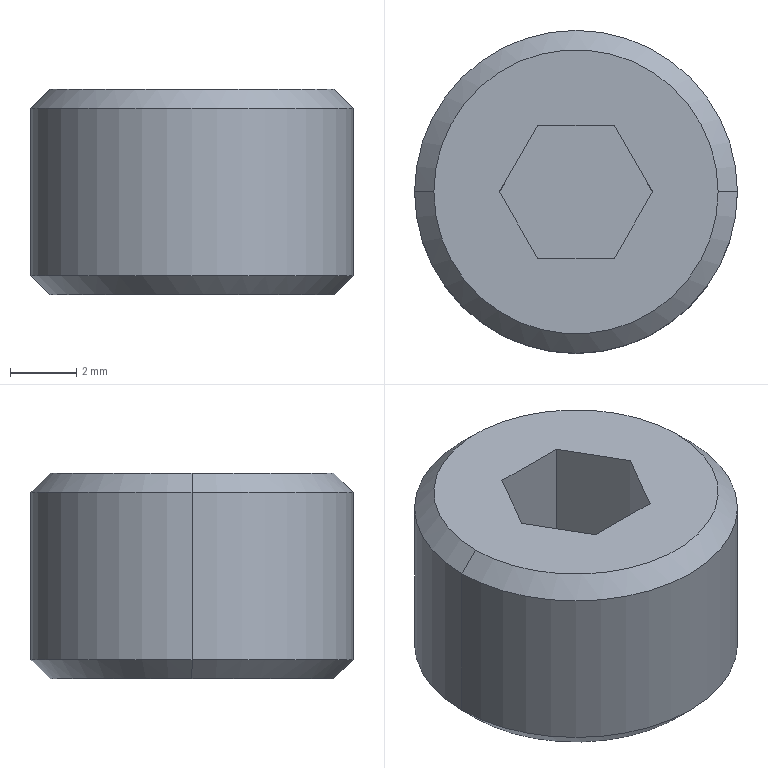Part | SolidWorks | features BaseBody 1 | 1 solid | 15 faces | box 9.728 x 9.728 x 6.2 mm | volume 395.486 mm3 | plane 9 | cone 4 | cylinder 2 | commonest cylinder face diameters 9.728 x2
STEP:
#1=CARTESIAN_POINT('',(-4.283,0.,-6.2));
#2=VERTEX_POINT('',#1);
#3=CARTESIAN_POINT('',(4.283,0.,-6.2));
#4=VERTEX_POINT('',#3);
#5=CARTESIAN_POINT('',(0.,0.,-6.2));
#6=DIRECTION('',(0.,0.,-1.));
#7=DIRECTION('',(-1.,0.,0.));
#8=AXIS2_PLACEMENT_3D('',#5,#6,#7);
#9=CIRCLE('',#8,4.283);
#10=EDGE_CURVE('',#2,#4,#9,.T.);
#11=ORIENTED_EDGE('',*,*,#10,.F.);
#12=CARTESIAN_POINT('',(-4.864,0.,-5.619));
#13=VERTEX_POINT('',#12);
#14=CARTESIAN_POINT('',(-4.864,0.,-5.619));
#15=DIRECTION('',(-0.7071,0.,0.7071));
#16=VECTOR('',#15,1000.);
#17=LINE('',#14,#16);
#18=EDGE_CURVE('',#2,#13,#17,.T.);
#19=ORIENTED_EDGE('',*,*,#18,.T.);
#20=CARTESIAN_POINT('',(4.864,0.,-5.619));
#21=VERTEX_POINT('',#20);
#22=CARTESIAN_POINT('',(0.,0.,-5.619));
#23=DIRECTION('',(0.,0.,-1.));
#24=DIRECTION('',(-1.,0.,0.));
#25=AXIS2_PLACEMENT_3D('',#22,#23,#24);
#26=CIRCLE('',#25,4.864);
#27=EDGE_CURVE('',#13,#21,#26,.T.);
#28=ORIENTED_EDGE('',*,*,#27,.T.);
#29=CARTESIAN_POINT('',(4.864,0.,-5.619));
#30=DIRECTION('',(0.7071,0.,0.7071));
#31=VECTOR('',#30,1000.);
#32=LINE('',#29,#31);
#33=EDGE_CURVE('',#4,#21,#32,.T.);
#34=ORIENTED_EDGE('',*,*,#33,.F.);
#35=EDGE_LOOP('',(#11,#19,#28,#34));
#36=FACE_OUTER_BOUND('',#35,.T.);
#37=CARTESIAN_POINT('',(0.,0.,-5.619));
#38=DIRECTION('',(0.,0.,1.));
#39=DIRECTION('',(1.,0.,0.));
#40=AXIS2_PLACEMENT_3D('',#37,#38,#39);
#41=CONICAL_SURFACE('',#40,4.864,0.7854);
#42=ADVANCED_FACE('',(#36),#41,.T.);
#43=CARTESIAN_POINT('',(-4.864,0.,-0.581));
#44=VERTEX_POINT('',#43);
#45=CARTESIAN_POINT('',(4.864,0.,-0.581));
#46=VERTEX_POINT('',#45);
#47=CARTESIAN_POINT('',(0.,0.,-0.581));
#48=DIRECTION('',(0.,0.,-1.));
#49=DIRECTION('',(-1.,0.,0.));
#50=AXIS2_PLACEMENT_3D('',#47,#48,#49);
#51=CIRCLE('',#50,4.864);
#52=EDGE_CURVE('',#44,#46,#51,.T.);
#53=ORIENTED_EDGE('',*,*,#52,.T.);
#54=CARTESIAN_POINT('',(4.864,0.,-6.2));
#55=DIRECTION('',(0.,0.,-1.));
#56=VECTOR('',#55,1000.);
#57=LINE('',#54,#56);
#58=EDGE_CURVE('',#46,#21,#57,.T.);
#59=ORIENTED_EDGE('',*,*,#58,.T.);
#60=ORIENTED_EDGE('',*,*,#27,.F.);
#61=CARTESIAN_POINT('',(-4.864,0.,-6.2));
#62=DIRECTION('',(0.,0.,-1.));
#63=VECTOR('',#62,1000.);
#64=LINE('',#61,#63);
#65=EDGE_CURVE('',#44,#13,#64,.T.);
#66=ORIENTED_EDGE('',*,*,#65,.F.);
#67=EDGE_LOOP('',(#53,#59,#60,#66));
#68=FACE_OUTER_BOUND('',#67,.T.);
#69=CARTESIAN_POINT('',(0.,0.,-6.2));
#70=DIRECTION('',(0.,0.,-1.));
#71=DIRECTION('',(-1.,0.,0.));
#72=AXIS2_PLACEMENT_3D('',#69,#70,#71);
#73=CYLINDRICAL_SURFACE('',#72,4.864);
#74=ADVANCED_FACE('',(#68),#73,.T.);
#75=CARTESIAN_POINT('',(-4.283,0.,0.));
#76=VERTEX_POINT('',#75);
#77=CARTESIAN_POINT('',(4.283,0.,0.));
#78=VERTEX_POINT('',#77);
#79=CARTESIAN_POINT('',(0.,0.,0.));
#80=DIRECTION('',(0.,0.,-1.));
#81=DIRECTION('',(-1.,0.,0.));
#82=AXIS2_PLACEMENT_3D('',#79,#80,#81);
#83=CIRCLE('',#82,4.283);
#84=EDGE_CURVE('',#76,#78,#83,.T.);
#85=ORIENTED_EDGE('',*,*,#84,.T.);
#86=CARTESIAN_POINT('',(4.283,0.,0.));
#87=DIRECTION('',(0.7071,0.,-0.7071));
#88=VECTOR('',#87,1000.);
#89=LINE('',#86,#88);
#90=EDGE_CURVE('',#78,#46,#89,.T.);
#91=ORIENTED_EDGE('',*,*,#90,.T.);
#92=ORIENTED_EDGE('',*,*,#52,.F.);
#93=CARTESIAN_POINT('',(-4.283,0.,0.));
#94=DIRECTION('',(-0.7071,0.,-0.7071));
#95=VECTOR('',#94,1000.);
#96=LINE('',#93,#95);
#97=EDGE_CURVE('',#76,#44,#96,.T.);
#98=ORIENTED_EDGE('',*,*,#97,.F.);
#99=EDGE_LOOP('',(#85,#91,#92,#98));
#100=FACE_OUTER_BOUND('',#99,.T.);
#101=CARTESIAN_POINT('',(0.,0.,0.));
#102=DIRECTION('',(0.,0.,-1.));
#103=DIRECTION('',(-1.,0.,0.));
#104=AXIS2_PLACEMENT_3D('',#101,#102,#103);
#105=CONICAL_SURFACE('',#104,4.283,0.7854);
#106=ADVANCED_FACE('',(#100),#105,.T.);
#107=ORIENTED_EDGE('',*,*,#84,.F.);
#108=CARTESIAN_POINT('',(0.,0.,0.));
#109=DIRECTION('',(0.,0.,-1.));
#110=DIRECTION('',(-1.,0.,0.));
#111=AXIS2_PLACEMENT_3D('',#108,#109,#110);
#112=CIRCLE('',#111,4.283);
#113=EDGE_CURVE('',#78,#76,#112,.T.);
#114=ORIENTED_EDGE('',*,*,#113,.F.);
#115=EDGE_LOOP('',(#107,#114));
#116=FACE_OUTER_BOUND('',#115,.T.);
#117=CARTESIAN_POINT('',(2.309,0.,0.));
#118=VERTEX_POINT('',#117);
#119=CARTESIAN_POINT('',(1.155,2.,0.));
#120=VERTEX_POINT('',#119);
#121=CARTESIAN_POINT('',(2.309,0.,0.));
#122=DIRECTION('',(-0.5,0.866,0.));
#123=VECTOR('',#122,1000.);
#124=LINE('',#121,#123);
#125=EDGE_CURVE('',#118,#120,#124,.T.);
#126=ORIENTED_EDGE('',*,*,#125,.F.);
#127=CARTESIAN_POINT('',(1.155,-2.,0.));
#128=VERTEX_POINT('',#127);
#129=CARTESIAN_POINT('',(1.155,-2.,0.));
#130=DIRECTION('',(0.5,0.866,0.));
#131=VECTOR('',#130,1000.);
#132=LINE('',#129,#131);
#133=EDGE_CURVE('',#128,#118,#132,.T.);
#134=ORIENTED_EDGE('',*,*,#133,.F.);
#135=CARTESIAN_POINT('',(-1.155,-2.,0.));
#136=VERTEX_POINT('',#135);
#137=CARTESIAN_POINT('',(-1.155,-2.,0.));
#138=DIRECTION('',(1.,0.,0.));
#139=VECTOR('',#138,1000.);
#140=LINE('',#137,#139);
#141=EDGE_CURVE('',#136,#128,#140,.T.);
#142=ORIENTED_EDGE('',*,*,#141,.F.);
#143=CARTESIAN_POINT('',(-2.309,0.,0.));
#144=VERTEX_POINT('',#143);
#145=CARTESIAN_POINT('',(-2.309,0.,0.));
#146=DIRECTION('',(0.5,-0.866,0.));
#147=VECTOR('',#146,1000.);
#148=LINE('',#145,#147);
#149=EDGE_CURVE('',#144,#136,#148,.T.);
#150=ORIENTED_EDGE('',*,*,#149,.F.);
#151=CARTESIAN_POINT('',(-1.155,2.,0.));
#152=VERTEX_POINT('',#151);
#153=CARTESIAN_POINT('',(-1.155,2.,0.));
#154=DIRECTION('',(-0.5,-0.866,0.));
#155=VECTOR('',#154,1000.);
#156=LINE('',#153,#155);
#157=EDGE_CURVE('',#152,#144,#156,.T.);
#158=ORIENTED_EDGE('',*,*,#157,.F.);
#159=CARTESIAN_POINT('',(-1.155,2.,0.));
#160=DIRECTION('',(1.,0.,0.));
#161=VECTOR('',#160,1000.);
#162=LINE('',#159,#161);
#163=EDGE_CURVE('',#152,#120,#162,.T.);
#164=ORIENTED_EDGE('',*,*,#163,.T.);
#165=EDGE_LOOP('',(#126,#134,#142,#150,#158,#164));
#166=FACE_BOUND('',#165,.T.);
#167=CARTESIAN_POINT('',(0.,0.,0.));
#168=DIRECTION('',(0.,0.,-1.));
#169=DIRECTION('',(-1.,0.,0.));
#170=AXIS2_PLACEMENT_3D('',#167,#168,#169);
#171=PLANE('',#170);
#172=ADVANCED_FACE('',(#116,#166),#171,.F.);
#173=ORIENTED_EDGE('',*,*,#90,.F.);
#174=ORIENTED_EDGE('',*,*,#113,.T.);
#175=ORIENTED_EDGE('',*,*,#97,.T.);
#176=CARTESIAN_POINT('',(0.,0.,-0.581));
#177=DIRECTION('',(0.,0.,-1.));
#178=DIRECTION('',(-1.,0.,0.));
#179=AXIS2_PLACEMENT_3D('',#176,#177,#178);
#180=CIRCLE('',#179,4.864);
#181=EDGE_CURVE('',#46,#44,#180,.T.);
#182=ORIENTED_EDGE('',*,*,#181,.F.);
#183=EDGE_LOOP('',(#173,#174,#175,#182));
#184=FACE_OUTER_BOUND('',#183,.T.);
#185=CARTESIAN_POINT('',(0.,0.,0.));
#186=DIRECTION('',(0.,0.,-1.));
#187=DIRECTION('',(-1.,0.,0.));
#188=AXIS2_PLACEMENT_3D('',#185,#186,#187);
#189=CONICAL_SURFACE('',#188,4.283,0.7854);
#190=ADVANCED_FACE('',(#184),#189,.T.);
#191=ORIENTED_EDGE('',*,*,#125,.T.);
#192=CARTESIAN_POINT('',(1.155,2.,-4.));
#193=VERTEX_POINT('',#192);
#194=CARTESIAN_POINT('',(1.155,2.,-4.));
#195=DIRECTION('',(0.,0.,1.));
#196=VECTOR('',#195,1000.);
#197=LINE('',#194,#196);
#198=EDGE_CURVE('',#193,#120,#197,.T.);
#199=ORIENTED_EDGE('',*,*,#198,.F.);
#200=CARTESIAN_POINT('',(2.309,0.,-4.));
#201=VERTEX_POINT('',#200);
#202=CARTESIAN_POINT('',(2.309,0.,-4.));
#203=DIRECTION('',(-0.5,0.866,0.));
#204=VECTOR('',#203,1000.);
#205=LINE('',#202,#204);
#206=EDGE_CURVE('',#201,#193,#205,.T.);
#207=ORIENTED_EDGE('',*,*,#206,.F.);
#208=CARTESIAN_POINT('',(2.309,0.,-4.));
#209=DIRECTION('',(0.,0.,1.));
#210=VECTOR('',#209,1000.);
#211=LINE('',#208,#210);
#212=EDGE_CURVE('',#201,#118,#211,.T.);
#213=ORIENTED_EDGE('',*,*,#212,.T.);
#214=EDGE_LOOP('',(#191,#199,#207,#213));
#215=FACE_OUTER_BOUND('',#214,.T.);
#216=CARTESIAN_POINT('',(2.309,0.,-4.));
#217=DIRECTION('',(0.866,0.5,0.));
#218=DIRECTION('',(-0.5,0.866,0.));
#219=AXIS2_PLACEMENT_3D('',#216,#217,#218);
#220=PLANE('',#219);
#221=ADVANCED_FACE('',(#215),#220,.F.);
#222=ORIENTED_EDGE('',*,*,#133,.T.);
#223=ORIENTED_EDGE('',*,*,#212,.F.);
#224=CARTESIAN_POINT('',(1.155,-2.,-4.));
#225=VERTEX_POINT('',#224);
#226=CARTESIAN_POINT('',(1.155,-2.,-4.));
#227=DIRECTION('',(0.5,0.866,0.));
#228=VECTOR('',#227,1000.);
#229=LINE('',#226,#228);
#230=EDGE_CURVE('',#225,#201,#229,.T.);
#231=ORIENTED_EDGE('',*,*,#230,.F.);
#232=CARTESIAN_POINT('',(1.155,-2.,-4.));
#233=DIRECTION('',(0.,0.,1.));
#234=VECTOR('',#233,1000.);
#235=LINE('',#232,#234);
#236=EDGE_CURVE('',#225,#128,#235,.T.);
#237=ORIENTED_EDGE('',*,*,#236,.T.);
#238=EDGE_LOOP('',(#222,#223,#231,#237));
#239=FACE_OUTER_BOUND('',#238,.T.);
#240=CARTESIAN_POINT('',(1.155,-2.,-4.));
#241=DIRECTION('',(0.866,-0.5,0.));
#242=DIRECTION('',(0.5,0.866,0.));
#243=AXIS2_PLACEMENT_3D('',#240,#241,#242);
#244=PLANE('',#243);
#245=ADVANCED_FACE('',(#239),#244,.F.);
#246=ORIENTED_EDGE('',*,*,#141,.T.);
#247=ORIENTED_EDGE('',*,*,#236,.F.);
#248=CARTESIAN_POINT('',(-1.155,-2.,-4.));
#249=VERTEX_POINT('',#248);
#250=CARTESIAN_POINT('',(-1.155,-2.,-4.));
#251=DIRECTION('',(1.,0.,0.));
#252=VECTOR('',#251,1000.);
#253=LINE('',#250,#252);
#254=EDGE_CURVE('',#249,#225,#253,.T.);
#255=ORIENTED_EDGE('',*,*,#254,.F.);
#256=CARTESIAN_POINT('',(-1.155,-2.,-4.));
#257=DIRECTION('',(0.,0.,1.));
#258=VECTOR('',#257,1000.);
#259=LINE('',#256,#258);
#260=EDGE_CURVE('',#249,#136,#259,.T.);
#261=ORIENTED_EDGE('',*,*,#260,.T.);
#262=EDGE_LOOP('',(#246,#247,#255,#261));
#263=FACE_OUTER_BOUND('',#262,.T.);
#264=CARTESIAN_POINT('',(-1.155,-2.,-4.));
#265=DIRECTION('',(0.,-1.,0.));
#266=DIRECTION('',(0.,0.,-1.));
#267=AXIS2_PLACEMENT_3D('',#264,#265,#266);
#268=PLANE('',#267);
#269=ADVANCED_FACE('',(#263),#268,.F.);
#270=ORIENTED_EDGE('',*,*,#149,.T.);
#271=ORIENTED_EDGE('',*,*,#260,.F.);
#272=CARTESIAN_POINT('',(-2.309,0.,-4.));
#273=VERTEX_POINT('',#272);
#274=CARTESIAN_POINT('',(-2.309,0.,-4.));
#275=DIRECTION('',(0.5,-0.866,0.));
#276=VECTOR('',#275,1000.);
#277=LINE('',#274,#276);
#278=EDGE_CURVE('',#273,#249,#277,.T.);
#279=ORIENTED_EDGE('',*,*,#278,.F.);
#280=CARTESIAN_POINT('',(-2.309,0.,-4.));
#281=DIRECTION('',(0.,0.,1.));
#282=VECTOR('',#281,1000.);
#283=LINE('',#280,#282);
#284=EDGE_CURVE('',#273,#144,#283,.T.);
#285=ORIENTED_EDGE('',*,*,#284,.T.);
#286=EDGE_LOOP('',(#270,#271,#279,#285));
#287=FACE_OUTER_BOUND('',#286,.T.);
#288=CARTESIAN_POINT('',(-2.309,0.,-4.));
#289=DIRECTION('',(-0.866,-0.5,0.));
#290=DIRECTION('',(0.5,-0.866,0.));
#291=AXIS2_PLACEMENT_3D('',#288,#289,#290);
#292=PLANE('',#291);
#293=ADVANCED_FACE('',(#287),#292,.F.);
#294=ORIENTED_EDGE('',*,*,#157,.T.);
#295=ORIENTED_EDGE('',*,*,#284,.F.);
#296=CARTESIAN_POINT('',(-1.155,2.,-4.));
#297=VERTEX_POINT('',#296);
#298=CARTESIAN_POINT('',(-1.155,2.,-4.));
#299=DIRECTION('',(-0.5,-0.866,0.));
#300=VECTOR('',#299,1000.);
#301=LINE('',#298,#300);
#302=EDGE_CURVE('',#297,#273,#301,.T.);
#303=ORIENTED_EDGE('',*,*,#302,.F.);
#304=CARTESIAN_POINT('',(-1.155,2.,-4.));
#305=DIRECTION('',(0.,0.,1.));
#306=VECTOR('',#305,1000.);
#307=LINE('',#304,#306);
#308=EDGE_CURVE('',#297,#152,#307,.T.);
#309=ORIENTED_EDGE('',*,*,#308,.T.);
#310=EDGE_LOOP('',(#294,#295,#303,#309));
#311=FACE_OUTER_BOUND('',#310,.T.);
#312=CARTESIAN_POINT('',(-1.155,2.,-4.));
#313=DIRECTION('',(-0.866,0.5,0.));
#314=DIRECTION('',(-0.5,-0.866,0.));
#315=AXIS2_PLACEMENT_3D('',#312,#313,#314);
#316=PLANE('',#315);
#317=ADVANCED_FACE('',(#311),#316,.F.);
#318=ORIENTED_EDGE('',*,*,#198,.T.);
#319=ORIENTED_EDGE('',*,*,#163,.F.);
#320=ORIENTED_EDGE('',*,*,#308,.F.);
#321=CARTESIAN_POINT('',(1.155,2.,-4.));
#322=DIRECTION('',(-1.,0.,0.));
#323=VECTOR('',#322,1000.);
#324=LINE('',#321,#323);
#325=EDGE_CURVE('',#193,#297,#324,.T.);
#326=ORIENTED_EDGE('',*,*,#325,.F.);
#327=EDGE_LOOP('',(#318,#319,#320,#326));
#328=FACE_OUTER_BOUND('',#327,.T.);
#329=CARTESIAN_POINT('',(1.155,2.,-4.));
#330=DIRECTION('',(0.,1.,0.));
#331=DIRECTION('',(0.,0.,1.));
#332=AXIS2_PLACEMENT_3D('',#329,#330,#331);
#333=PLANE('',#332);
#334=ADVANCED_FACE('',(#328),#333,.F.);
#335=ORIENTED_EDGE('',*,*,#58,.F.);
#336=ORIENTED_EDGE('',*,*,#181,.T.);
#337=ORIENTED_EDGE('',*,*,#65,.T.);
#338=CARTESIAN_POINT('',(0.,0.,-5.619));
#339=DIRECTION('',(0.,0.,-1.));
#340=DIRECTION('',(-1.,0.,0.));
#341=AXIS2_PLACEMENT_3D('',#338,#339,#340);
#342=CIRCLE('',#341,4.864);
#343=EDGE_CURVE('',#21,#13,#342,.T.);
#344=ORIENTED_EDGE('',*,*,#343,.F.);
#345=EDGE_LOOP('',(#335,#336,#337,#344));
#346=FACE_OUTER_BOUND('',#345,.T.);
#347=CARTESIAN_POINT('',(0.,0.,-6.2));
#348=DIRECTION('',(0.,0.,-1.));
#349=DIRECTION('',(-1.,0.,0.));
#350=AXIS2_PLACEMENT_3D('',#347,#348,#349);
#351=CYLINDRICAL_SURFACE('',#350,4.864);
#352=ADVANCED_FACE('',(#346),#351,.T.);
#353=ORIENTED_EDGE('',*,*,#254,.T.);
#354=ORIENTED_EDGE('',*,*,#230,.T.);
#355=ORIENTED_EDGE('',*,*,#206,.T.);
#356=ORIENTED_EDGE('',*,*,#325,.T.);
#357=ORIENTED_EDGE('',*,*,#302,.T.);
#358=ORIENTED_EDGE('',*,*,#278,.T.);
#359=EDGE_LOOP('',(#353,#354,#355,#356,#357,#358));
#360=FACE_OUTER_BOUND('',#359,.T.);
#361=CARTESIAN_POINT('',(0.,0.,-4.));
#362=DIRECTION('',(0.,0.,1.));
#363=DIRECTION('',(1.,0.,0.));
#364=AXIS2_PLACEMENT_3D('',#361,#362,#363);
#365=PLANE('',#364);
#366=ADVANCED_FACE('',(#360),#365,.T.);
#367=ORIENTED_EDGE('',*,*,#18,.F.);
#368=CARTESIAN_POINT('',(0.,0.,-6.2));
#369=DIRECTION('',(0.,0.,-1.));
#370=DIRECTION('',(-1.,0.,0.));
#371=AXIS2_PLACEMENT_3D('',#368,#369,#370);
#372=CIRCLE('',#371,4.283);
#373=EDGE_CURVE('',#4,#2,#372,.T.);
#374=ORIENTED_EDGE('',*,*,#373,.F.);
#375=ORIENTED_EDGE('',*,*,#33,.T.);
#376=ORIENTED_EDGE('',*,*,#343,.T.);
#377=EDGE_LOOP('',(#367,#374,#375,#376));
#378=FACE_OUTER_BOUND('',#377,.T.);
#379=CARTESIAN_POINT('',(0.,0.,-5.619));
#380=DIRECTION('',(0.,0.,1.));
#381=DIRECTION('',(1.,0.,0.));
#382=AXIS2_PLACEMENT_3D('',#379,#380,#381);
#383=CONICAL_SURFACE('',#382,4.864,0.7854);
#384=ADVANCED_FACE('',(#378),#383,.T.);
#385=ORIENTED_EDGE('',*,*,#373,.T.);
#386=ORIENTED_EDGE('',*,*,#10,.T.);
#387=EDGE_LOOP('',(#385,#386));
#388=FACE_OUTER_BOUND('',#387,.T.);
#389=CARTESIAN_POINT('',(0.,4.283,-6.2));
#390=DIRECTION('',(0.,0.,1.));
#391=DIRECTION('',(1.,0.,0.));
#392=AXIS2_PLACEMENT_3D('',#389,#390,#391);
#393=PLANE('',#392);
#394=ADVANCED_FACE('',(#388),#393,.F.);
#395=CLOSED_SHELL('',(#42,#74,#106,#172,#190,#221,#245,#269,#293,#317,#334,#352,#366,#384,#394));
#396=MANIFOLD_SOLID_BREP('',#395);
#397=CARTESIAN_POINT('',(0.,0.,0.));
#398=DIRECTION('',(0.,0.,1.));
#399=DIRECTION('',(1.,0.,0.));
#400=AXIS2_PLACEMENT_3D('',#397,#398,#399);
#401=(LENGTH_UNIT()NAMED_UNIT(*)SI_UNIT(.MILLI.,.METRE.));
#402=UNCERTAINTY_MEASURE_WITH_UNIT(LENGTH_MEASURE(0.00001),#401,'','');
#403=(NAMED_UNIT(*)PLANE_ANGLE_UNIT()SI_UNIT($,.RADIAN.));
#404=(NAMED_UNIT(*)SI_UNIT($,.STERADIAN.)SOLID_ANGLE_UNIT());
#405=(GEOMETRIC_REPRESENTATION_CONTEXT(3)GLOBAL_UNCERTAINTY_ASSIGNED_CONTEXT((#402))GLOBAL_UNIT_ASSIGNED_CONTEXT((#401,#403,#404))REPRESENTATION_CONTEXT('',''));
#406=ADVANCED_BREP_SHAPE_REPRESENTATION('',(#396,#400),#405);